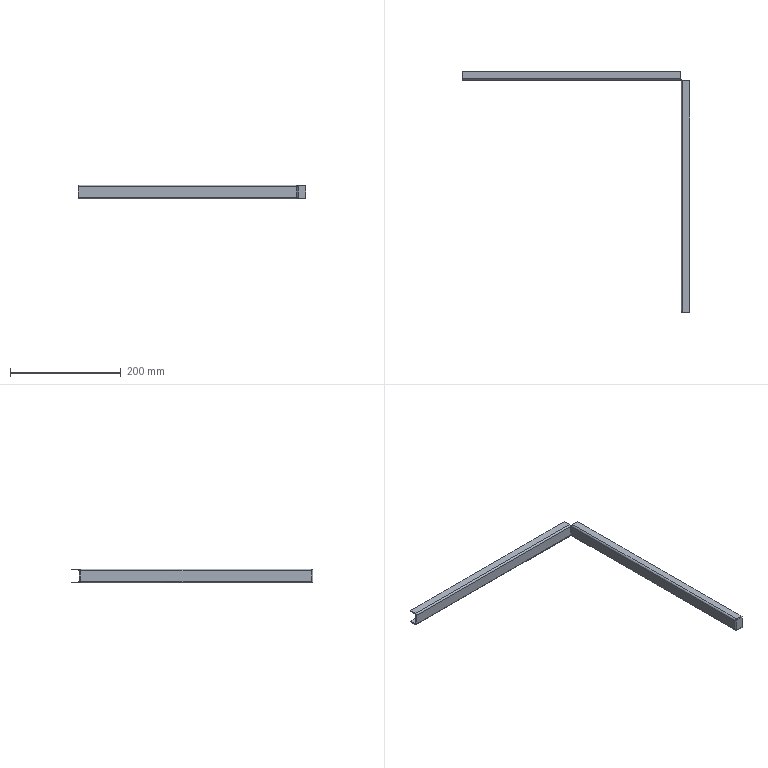Part | NX | features solid 2 | 1 solid | 50 faces | box 411 x 436 x 25 mm | volume 63952 mm3 | plane 38 | cylinder 12 | commonest cylinder face diameters 3 x6 6 x6
STEP:
#1=CARTESIAN_POINT('',(1095.5,89.,905.9));
#2=VERTEX_POINT('',#1);
#3=CARTESIAN_POINT('',(1095.5,89.,884.1));
#4=VERTEX_POINT('',#3);
#5=CARTESIAN_POINT('',(1095.5,89.,904.5));
#6=DIRECTION('',(0.,0.,-1.));
#7=VECTOR('',#6,1000.);
#8=LINE('',#5,#7);
#9=EDGE_CURVE('',#2,#4,#8,.T.);
#10=ORIENTED_EDGE('',*,*,#9,.F.);
#11=CARTESIAN_POINT('',(1108.5,89.,905.9));
#12=VERTEX_POINT('',#11);
#13=CARTESIAN_POINT('',(1093.851,89.,905.9));
#14=DIRECTION('',(-1.,0.,0.));
#15=VECTOR('',#14,1000.);
#16=LINE('',#13,#15);
#17=EDGE_CURVE('',#12,#2,#16,.T.);
#18=ORIENTED_EDGE('',*,*,#17,.F.);
#19=CARTESIAN_POINT('',(1108.5,89.,884.1));
#20=VERTEX_POINT('',#19);
#21=CARTESIAN_POINT('',(1108.5,89.,885.5));
#22=DIRECTION('',(0.,0.,1.));
#23=VECTOR('',#22,1000.);
#24=LINE('',#21,#23);
#25=EDGE_CURVE('',#20,#12,#24,.T.);
#26=ORIENTED_EDGE('',*,*,#25,.F.);
#27=CARTESIAN_POINT('',(1093.851,89.,884.1));
#28=DIRECTION('',(1.,0.,0.));
#29=VECTOR('',#28,1000.);
#30=LINE('',#27,#29);
#31=EDGE_CURVE('',#4,#20,#30,.T.);
#32=ORIENTED_EDGE('',*,*,#31,.F.);
#33=EDGE_LOOP('',(#10,#18,#26,#32));
#34=FACE_BOUND('',#33,.T.);
#35=CARTESIAN_POINT('',(895.,89.,895.));
#36=DIRECTION('',(0.,-1.,0.));
#37=DIRECTION('',(-1.,0.,0.));
#38=AXIS2_PLACEMENT_3D('',#35,#36,#37);
#39=PLANE('',#38);
#40=ADVANCED_FACE('',(#34),#39,.F.);
#41=CARTESIAN_POINT('',(1108.5,87.5,905.9));
#42=VERTEX_POINT('',#41);
#43=CARTESIAN_POINT('',(1095.5,87.5,905.9));
#44=VERTEX_POINT('',#43);
#45=CARTESIAN_POINT('',(1093.851,87.5,905.9));
#46=DIRECTION('',(-1.,0.,0.));
#47=VECTOR('',#46,1000.);
#48=LINE('',#45,#47);
#49=EDGE_CURVE('',#42,#44,#48,.T.);
#50=ORIENTED_EDGE('',*,*,#49,.T.);
#51=CARTESIAN_POINT('',(1095.5,87.5,884.1));
#52=VERTEX_POINT('',#51);
#53=CARTESIAN_POINT('',(1095.5,87.5,904.5));
#54=DIRECTION('',(0.,0.,-1.));
#55=VECTOR('',#54,1000.);
#56=LINE('',#53,#55);
#57=EDGE_CURVE('',#44,#52,#56,.T.);
#58=ORIENTED_EDGE('',*,*,#57,.T.);
#59=CARTESIAN_POINT('',(1108.5,87.5,884.1));
#60=VERTEX_POINT('',#59);
#61=CARTESIAN_POINT('',(1093.851,87.5,884.1));
#62=DIRECTION('',(1.,0.,0.));
#63=VECTOR('',#62,1000.);
#64=LINE('',#61,#63);
#65=EDGE_CURVE('',#52,#60,#64,.T.);
#66=ORIENTED_EDGE('',*,*,#65,.T.);
#67=CARTESIAN_POINT('',(1108.5,87.5,885.5));
#68=DIRECTION('',(0.,0.,1.));
#69=VECTOR('',#68,1000.);
#70=LINE('',#67,#69);
#71=EDGE_CURVE('',#60,#42,#70,.T.);
#72=ORIENTED_EDGE('',*,*,#71,.T.);
#73=EDGE_LOOP('',(#50,#58,#66,#72));
#74=FACE_BOUND('',#73,.T.);
#75=CARTESIAN_POINT('',(895.,87.5,895.));
#76=DIRECTION('',(0.,-1.,0.));
#77=DIRECTION('',(-1.,0.,0.));
#78=AXIS2_PLACEMENT_3D('',#75,#76,#77);
#79=PLANE('',#78);
#80=ADVANCED_FACE('',(#74),#79,.T.);
#81=ORIENTED_EDGE('',*,*,#25,.T.);
#82=CARTESIAN_POINT('',(1108.5,87.5,905.9));
#83=DIRECTION('',(0.,1.,0.));
#84=VECTOR('',#83,1000.);
#85=LINE('',#82,#84);
#86=EDGE_CURVE('',#42,#12,#85,.T.);
#87=ORIENTED_EDGE('',*,*,#86,.F.);
#88=ORIENTED_EDGE('',*,*,#71,.F.);
#89=CARTESIAN_POINT('',(1108.5,87.5,884.1));
#90=DIRECTION('',(0.,1.,0.));
#91=VECTOR('',#90,1000.);
#92=LINE('',#89,#91);
#93=EDGE_CURVE('',#60,#20,#92,.T.);
#94=ORIENTED_EDGE('',*,*,#93,.T.);
#95=EDGE_LOOP('',(#81,#87,#88,#94));
#96=FACE_BOUND('',#95,.T.);
#97=CARTESIAN_POINT('',(1108.5,87.5,885.5));
#98=DIRECTION('',(-1.,0.,0.));
#99=DIRECTION('',(0.,0.,1.));
#100=AXIS2_PLACEMENT_3D('',#97,#98,#99);
#101=PLANE('',#100);
#102=ADVANCED_FACE('',(#96),#101,.F.);
#103=CARTESIAN_POINT('',(1094.,90.5,885.5));
#104=VERTEX_POINT('',#103);
#105=CARTESIAN_POINT('',(1095.5,89.,884.1));
#106=CARTESIAN_POINT('',(1094.621,89.,884.1));
#107=CARTESIAN_POINT('',(1094.,89.621,884.68));
#108=CARTESIAN_POINT('',(1094.,90.5,885.5));
#109=(BOUNDED_CURVE()B_SPLINE_CURVE(3,(#105,#106,#107,#108),.UNSPECIFIED.,.F.,.F.)B_SPLINE_CURVE_WITH_KNOTS((4,4),(3.142,4.712),.PIECEWISE_BEZIER_KNOTS.)CURVE()GEOMETRIC_REPRESENTATION_ITEM()RATIONAL_B_SPLINE_CURVE((1.,0.8047,0.8047,1.))REPRESENTATION_ITEM(''));
#110=EDGE_CURVE('',#4,#104,#109,.T.);
#111=ORIENTED_EDGE('',*,*,#110,.F.);
#112=CARTESIAN_POINT('',(1092.902,89.,884.1));
#113=VERTEX_POINT('',#112);
#114=CARTESIAN_POINT('',(2092.5,89.,884.1));
#115=DIRECTION('',(1.,0.,0.));
#116=VECTOR('',#115,1000.);
#117=LINE('',#114,#116);
#118=EDGE_CURVE('',#113,#4,#117,.T.);
#119=ORIENTED_EDGE('',*,*,#118,.F.);
#120=CARTESIAN_POINT('',(1092.5,90.5,885.5));
#121=VERTEX_POINT('',#120);
#122=CARTESIAN_POINT('',(1092.902,89.,884.1));
#123=CARTESIAN_POINT('',(1092.637,89.459,884.528));
#124=CARTESIAN_POINT('',(1092.5,89.97,885.006));
#125=CARTESIAN_POINT('',(1092.5,90.5,885.5));
#126=(BOUNDED_CURVE()B_SPLINE_CURVE(3,(#122,#123,#124,#125),.UNSPECIFIED.,.F.,.F.)B_SPLINE_CURVE_WITH_KNOTS((4,4),(4.189,4.712),.PIECEWISE_BEZIER_KNOTS.)CURVE()GEOMETRIC_REPRESENTATION_ITEM()RATIONAL_B_SPLINE_CURVE((1.,0.9773,0.9773,1.))REPRESENTATION_ITEM(''));
#127=EDGE_CURVE('',#113,#121,#126,.T.);
#128=ORIENTED_EDGE('',*,*,#127,.T.);
#129=CARTESIAN_POINT('',(1094.,90.5,885.5));
#130=DIRECTION('',(-1.,0.,0.));
#131=VECTOR('',#130,1000.);
#132=LINE('',#129,#131);
#133=EDGE_CURVE('',#104,#121,#132,.T.);
#134=ORIENTED_EDGE('',*,*,#133,.F.);
#135=EDGE_LOOP('',(#111,#119,#128,#134));
#136=FACE_BOUND('',#135,.T.);
#137=CARTESIAN_POINT('',(92.5,821.555,1567.818));
#138=DIRECTION('',(0.,-0.6823,0.7311));
#139=DIRECTION('',(-1.,0.,0.));
#140=AXIS2_PLACEMENT_3D('',#137,#138,#139);
#141=PLANE('',#140);
#142=ADVANCED_FACE('',(#136),#141,.F.);
#143=ORIENTED_EDGE('',*,*,#118,.T.);
#144=ORIENTED_EDGE('',*,*,#31,.T.);
#145=ORIENTED_EDGE('',*,*,#93,.F.);
#146=ORIENTED_EDGE('',*,*,#65,.F.);
#147=CARTESIAN_POINT('',(1095.5,90.5,884.1));
#148=DIRECTION('',(0.,0.,-1.));
#149=DIRECTION('',(0.,1.,0.));
#150=AXIS2_PLACEMENT_3D('',#147,#148,#149);
#151=CIRCLE('',#150,3.);
#152=EDGE_CURVE('',#52,#113,#151,.T.);
#153=ORIENTED_EDGE('',*,*,#152,.T.);
#154=EDGE_LOOP('',(#143,#144,#145,#146,#153));
#155=FACE_BOUND('',#154,.T.);
#156=CARTESIAN_POINT('',(92.5,89.,884.1));
#157=DIRECTION('',(0.,0.,1.));
#158=DIRECTION('',(0.,-1.,0.));
#159=AXIS2_PLACEMENT_3D('',#156,#157,#158);
#160=PLANE('',#159);
#161=ADVANCED_FACE('',(#155),#160,.F.);
#162=CARTESIAN_POINT('',(1092.902,89.,905.9));
#163=VERTEX_POINT('',#162);
#164=CARTESIAN_POINT('',(1092.5,90.5,904.5));
#165=VERTEX_POINT('',#164);
#166=CARTESIAN_POINT('',(1092.902,89.,905.9));
#167=CARTESIAN_POINT('',(1092.637,89.459,905.472));
#168=CARTESIAN_POINT('',(1092.5,89.97,904.994));
#169=CARTESIAN_POINT('',(1092.5,90.5,904.5));
#170=(BOUNDED_CURVE()B_SPLINE_CURVE(3,(#166,#167,#168,#169),.UNSPECIFIED.,.F.,.F.)B_SPLINE_CURVE_WITH_KNOTS((4,4),(1.047,1.571),.PIECEWISE_BEZIER_KNOTS.)CURVE()GEOMETRIC_REPRESENTATION_ITEM()RATIONAL_B_SPLINE_CURVE((1.,0.9773,0.9773,1.))REPRESENTATION_ITEM(''));
#171=EDGE_CURVE('',#163,#165,#170,.T.);
#172=ORIENTED_EDGE('',*,*,#171,.F.);
#173=CARTESIAN_POINT('',(2092.5,89.,905.9));
#174=DIRECTION('',(1.,0.,0.));
#175=VECTOR('',#174,1000.);
#176=LINE('',#173,#175);
#177=EDGE_CURVE('',#163,#2,#176,.T.);
#178=ORIENTED_EDGE('',*,*,#177,.T.);
#179=CARTESIAN_POINT('',(1094.,90.5,904.5));
#180=VERTEX_POINT('',#179);
#181=CARTESIAN_POINT('',(1095.5,89.,905.9));
#182=CARTESIAN_POINT('',(1094.621,89.,905.9));
#183=CARTESIAN_POINT('',(1094.,89.621,905.32));
#184=CARTESIAN_POINT('',(1094.,90.5,904.5));
#185=(BOUNDED_CURVE()B_SPLINE_CURVE(3,(#181,#182,#183,#184),.UNSPECIFIED.,.F.,.F.)B_SPLINE_CURVE_WITH_KNOTS((4,4),(0.,1.571),.PIECEWISE_BEZIER_KNOTS.)CURVE()GEOMETRIC_REPRESENTATION_ITEM()RATIONAL_B_SPLINE_CURVE((1.,0.8047,0.8047,1.))REPRESENTATION_ITEM(''));
#186=EDGE_CURVE('',#2,#180,#185,.T.);
#187=ORIENTED_EDGE('',*,*,#186,.T.);
#188=CARTESIAN_POINT('',(1094.,90.5,904.5));
#189=DIRECTION('',(-1.,0.,0.));
#190=VECTOR('',#189,1000.);
#191=LINE('',#188,#190);
#192=EDGE_CURVE('',#180,#165,#191,.T.);
#193=ORIENTED_EDGE('',*,*,#192,.T.);
#194=EDGE_LOOP('',(#172,#178,#187,#193));
#195=FACE_BOUND('',#194,.T.);
#196=CARTESIAN_POINT('',(92.5,821.555,222.182));
#197=DIRECTION('',(0.,0.6823,0.7311));
#198=DIRECTION('',(1.,0.,0.));
#199=AXIS2_PLACEMENT_3D('',#196,#197,#198);
#200=PLANE('',#199);
#201=ADVANCED_FACE('',(#195),#200,.T.);
#202=ORIENTED_EDGE('',*,*,#127,.F.);
#203=ORIENTED_EDGE('',*,*,#152,.F.);
#204=ORIENTED_EDGE('',*,*,#57,.F.);
#205=CARTESIAN_POINT('',(1095.5,90.5,905.9));
#206=DIRECTION('',(0.,0.,-1.));
#207=DIRECTION('',(0.,1.,0.));
#208=AXIS2_PLACEMENT_3D('',#205,#206,#207);
#209=CIRCLE('',#208,3.);
#210=EDGE_CURVE('',#44,#163,#209,.T.);
#211=ORIENTED_EDGE('',*,*,#210,.T.);
#212=ORIENTED_EDGE('',*,*,#171,.T.);
#213=CARTESIAN_POINT('',(1092.5,90.5,885.5));
#214=DIRECTION('',(0.,0.,1.));
#215=VECTOR('',#214,1000.);
#216=LINE('',#213,#215);
#217=EDGE_CURVE('',#121,#165,#216,.T.);
#218=ORIENTED_EDGE('',*,*,#217,.F.);
#219=EDGE_LOOP('',(#202,#203,#204,#211,#212,#218));
#220=FACE_BOUND('',#219,.T.);
#221=CARTESIAN_POINT('',(1095.5,90.5,885.5));
#222=DIRECTION('',(0.,0.,1.));
#223=DIRECTION('',(1.,0.,0.));
#224=AXIS2_PLACEMENT_3D('',#221,#222,#223);
#225=CYLINDRICAL_SURFACE('',#224,3.);
#226=ADVANCED_FACE('',(#220),#225,.T.);
#227=ORIENTED_EDGE('',*,*,#210,.F.);
#228=ORIENTED_EDGE('',*,*,#49,.F.);
#229=ORIENTED_EDGE('',*,*,#86,.T.);
#230=ORIENTED_EDGE('',*,*,#17,.T.);
#231=ORIENTED_EDGE('',*,*,#177,.F.);
#232=EDGE_LOOP('',(#227,#228,#229,#230,#231));
#233=FACE_BOUND('',#232,.T.);
#234=CARTESIAN_POINT('',(92.5,89.,905.9));
#235=DIRECTION('',(0.,0.,1.));
#236=DIRECTION('',(0.,-1.,0.));
#237=AXIS2_PLACEMENT_3D('',#234,#235,#236);
#238=PLANE('',#237);
#239=ADVANCED_FACE('',(#233),#238,.T.);
#240=ORIENTED_EDGE('',*,*,#9,.T.);
#241=ORIENTED_EDGE('',*,*,#110,.T.);
#242=CARTESIAN_POINT('',(1094.,90.5,885.5));
#243=DIRECTION('',(0.,0.,1.));
#244=VECTOR('',#243,1000.);
#245=LINE('',#242,#244);
#246=EDGE_CURVE('',#104,#180,#245,.T.);
#247=ORIENTED_EDGE('',*,*,#246,.T.);
#248=ORIENTED_EDGE('',*,*,#186,.F.);
#249=EDGE_LOOP('',(#240,#241,#247,#248));
#250=FACE_BOUND('',#249,.T.);
#251=CARTESIAN_POINT('',(1095.5,90.5,885.5));
#252=DIRECTION('',(0.,0.,1.));
#253=DIRECTION('',(1.,0.,0.));
#254=AXIS2_PLACEMENT_3D('',#251,#252,#253);
#255=CYLINDRICAL_SURFACE('',#254,1.5);
#256=ADVANCED_FACE('',(#250),#255,.F.);
#257=CARTESIAN_POINT('',(1108.5,506.,884.));
#258=VERTEX_POINT('',#257);
#259=CARTESIAN_POINT('',(1095.5,506.,884.));
#260=VERTEX_POINT('',#259);
#261=CARTESIAN_POINT('',(1108.5,506.,884.));
#262=DIRECTION('',(-1.,0.,0.));
#263=VECTOR('',#262,1000.);
#264=LINE('',#261,#263);
#265=EDGE_CURVE('',#258,#260,#264,.T.);
#266=ORIENTED_EDGE('',*,*,#265,.T.);
#267=CARTESIAN_POINT('',(1095.5,89.1,884.));
#268=VERTEX_POINT('',#267);
#269=CARTESIAN_POINT('',(1095.5,87.5,884.));
#270=DIRECTION('',(0.,1.,0.));
#271=VECTOR('',#270,1000.);
#272=LINE('',#269,#271);
#273=EDGE_CURVE('',#268,#260,#272,.T.);
#274=ORIENTED_EDGE('',*,*,#273,.F.);
#275=CARTESIAN_POINT('',(1095.5,87.5,884.));
#276=VERTEX_POINT('',#275);
#277=CARTESIAN_POINT('',(1095.5,87.5,884.));
#278=DIRECTION('',(0.,1.,0.));
#279=VECTOR('',#278,1000.);
#280=LINE('',#277,#279);
#281=EDGE_CURVE('',#276,#268,#280,.T.);
#282=ORIENTED_EDGE('',*,*,#281,.F.);
#283=CARTESIAN_POINT('',(1108.5,87.5,884.));
#284=VERTEX_POINT('',#283);
#285=CARTESIAN_POINT('',(1108.5,87.5,884.));
#286=DIRECTION('',(-1.,0.,0.));
#287=VECTOR('',#286,1000.);
#288=LINE('',#285,#287);
#289=EDGE_CURVE('',#284,#276,#288,.T.);
#290=ORIENTED_EDGE('',*,*,#289,.F.);
#291=CARTESIAN_POINT('',(1108.5,87.5,884.));
#292=DIRECTION('',(0.,1.,0.));
#293=VECTOR('',#292,1000.);
#294=LINE('',#291,#293);
#295=EDGE_CURVE('',#284,#258,#294,.T.);
#296=ORIENTED_EDGE('',*,*,#295,.T.);
#297=EDGE_LOOP('',(#266,#274,#282,#290,#296));
#298=FACE_BOUND('',#297,.T.);
#299=CARTESIAN_POINT('',(1108.5,87.5,884.));
#300=DIRECTION('',(0.,0.,-1.));
#301=DIRECTION('',(-1.,0.,0.));
#302=AXIS2_PLACEMENT_3D('',#299,#300,#301);
#303=PLANE('',#302);
#304=ADVANCED_FACE('',(#298),#303,.F.);
#305=CARTESIAN_POINT('',(1108.5,506.,882.5));
#306=VERTEX_POINT('',#305);
#307=CARTESIAN_POINT('',(1095.5,506.,882.5));
#308=VERTEX_POINT('',#307);
#309=CARTESIAN_POINT('',(1108.5,506.,882.5));
#310=DIRECTION('',(-1.,0.,0.));
#311=VECTOR('',#310,1000.);
#312=LINE('',#309,#311);
#313=EDGE_CURVE('',#306,#308,#312,.T.);
#314=ORIENTED_EDGE('',*,*,#313,.F.);
#315=CARTESIAN_POINT('',(1108.5,87.5,882.5));
#316=VERTEX_POINT('',#315);
#317=CARTESIAN_POINT('',(1108.5,87.5,882.5));
#318=DIRECTION('',(0.,1.,0.));
#319=VECTOR('',#318,1000.);
#320=LINE('',#317,#319);
#321=EDGE_CURVE('',#316,#306,#320,.T.);
#322=ORIENTED_EDGE('',*,*,#321,.F.);
#323=CARTESIAN_POINT('',(1095.5,87.5,882.5));
#324=VERTEX_POINT('',#323);
#325=CARTESIAN_POINT('',(1108.5,87.5,882.5));
#326=DIRECTION('',(-1.,0.,0.));
#327=VECTOR('',#326,1000.);
#328=LINE('',#325,#327);
#329=EDGE_CURVE('',#316,#324,#328,.T.);
#330=ORIENTED_EDGE('',*,*,#329,.T.);
#331=CARTESIAN_POINT('',(1095.5,89.1,882.5));
#332=VERTEX_POINT('',#331);
#333=CARTESIAN_POINT('',(1095.5,87.5,882.5));
#334=DIRECTION('',(0.,1.,0.));
#335=VECTOR('',#334,1000.);
#336=LINE('',#333,#335);
#337=EDGE_CURVE('',#324,#332,#336,.T.);
#338=ORIENTED_EDGE('',*,*,#337,.T.);
#339=CARTESIAN_POINT('',(1095.5,87.5,882.5));
#340=DIRECTION('',(0.,1.,0.));
#341=VECTOR('',#340,1000.);
#342=LINE('',#339,#341);
#343=EDGE_CURVE('',#332,#308,#342,.T.);
#344=ORIENTED_EDGE('',*,*,#343,.T.);
#345=EDGE_LOOP('',(#314,#322,#330,#338,#344));
#346=FACE_BOUND('',#345,.T.);
#347=CARTESIAN_POINT('',(1108.5,87.5,882.5));
#348=DIRECTION('',(0.,0.,-1.));
#349=DIRECTION('',(-1.,0.,0.));
#350=AXIS2_PLACEMENT_3D('',#347,#348,#349);
#351=PLANE('',#350);
#352=ADVANCED_FACE('',(#346),#351,.T.);
#353=CARTESIAN_POINT('',(1095.5,87.5,882.5));
#354=DIRECTION('',(0.,0.,1.));
#355=VECTOR('',#354,1000.);
#356=LINE('',#353,#355);
#357=EDGE_CURVE('',#324,#276,#356,.T.);
#358=ORIENTED_EDGE('',*,*,#357,.F.);
#359=ORIENTED_EDGE('',*,*,#329,.F.);
#360=CARTESIAN_POINT('',(1108.5,87.5,882.5));
#361=DIRECTION('',(0.,0.,-1.));
#362=VECTOR('',#361,1000.);
#363=LINE('',#360,#362);
#364=EDGE_CURVE('',#284,#316,#363,.T.);
#365=ORIENTED_EDGE('',*,*,#364,.F.);
#366=ORIENTED_EDGE('',*,*,#289,.T.);
#367=EDGE_LOOP('',(#358,#359,#365,#366));
#368=FACE_BOUND('',#367,.T.);
#369=CARTESIAN_POINT('',(1092.5,87.5,882.5));
#370=DIRECTION('',(0.,1.,0.));
#371=DIRECTION('',(1.,0.,0.));
#372=AXIS2_PLACEMENT_3D('',#369,#370,#371);
#373=PLANE('',#372);
#374=ADVANCED_FACE('',(#368),#373,.F.);
#375=ORIENTED_EDGE('',*,*,#295,.F.);
#376=ORIENTED_EDGE('',*,*,#364,.T.);
#377=ORIENTED_EDGE('',*,*,#321,.T.);
#378=CARTESIAN_POINT('',(1108.5,506.,882.5));
#379=DIRECTION('',(0.,0.,-1.));
#380=VECTOR('',#379,1000.);
#381=LINE('',#378,#380);
#382=EDGE_CURVE('',#258,#306,#381,.T.);
#383=ORIENTED_EDGE('',*,*,#382,.F.);
#384=EDGE_LOOP('',(#375,#376,#377,#383));
#385=FACE_BOUND('',#384,.T.);
#386=CARTESIAN_POINT('',(1108.5,87.5,882.5));
#387=DIRECTION('',(-1.,0.,0.));
#388=DIRECTION('',(0.,1.,0.));
#389=AXIS2_PLACEMENT_3D('',#386,#387,#388);
#390=PLANE('',#389);
#391=ADVANCED_FACE('',(#385),#390,.F.);
#392=ORIENTED_EDGE('',*,*,#281,.T.);
#393=CARTESIAN_POINT('',(1095.5,89.1,895.));
#394=DIRECTION('',(0.,0.,-1.));
#395=VECTOR('',#394,1000.);
#396=LINE('',#393,#395);
#397=EDGE_CURVE('',#268,#332,#396,.T.);
#398=ORIENTED_EDGE('',*,*,#397,.T.);
#399=ORIENTED_EDGE('',*,*,#337,.F.);
#400=ORIENTED_EDGE('',*,*,#357,.T.);
#401=EDGE_LOOP('',(#392,#398,#399,#400));
#402=FACE_BOUND('',#401,.T.);
#403=CARTESIAN_POINT('',(1095.5,87.5,882.5));
#404=DIRECTION('',(1.,0.,0.));
#405=DIRECTION('',(0.,-1.,0.));
#406=AXIS2_PLACEMENT_3D('',#403,#404,#405);
#407=PLANE('',#406);
#408=ADVANCED_FACE('',(#402),#407,.F.);
#409=CARTESIAN_POINT('',(1092.902,89.1,884.));
#410=VERTEX_POINT('',#409);
#411=CARTESIAN_POINT('',(1095.5,89.1,885.5));
#412=DIRECTION('',(0.,1.,0.));
#413=DIRECTION('',(0.,0.,1.));
#414=AXIS2_PLACEMENT_3D('',#411,#412,#413);
#415=CIRCLE('',#414,3.);
#416=EDGE_CURVE('',#332,#410,#415,.T.);
#417=ORIENTED_EDGE('',*,*,#416,.F.);
#418=ORIENTED_EDGE('',*,*,#397,.F.);
#419=CARTESIAN_POINT('',(2092.5,89.1,884.));
#420=DIRECTION('',(1.,0.,0.));
#421=VECTOR('',#420,1000.);
#422=LINE('',#419,#421);
#423=EDGE_CURVE('',#410,#268,#422,.T.);
#424=ORIENTED_EDGE('',*,*,#423,.F.);
#425=EDGE_LOOP('',(#417,#418,#424));
#426=FACE_BOUND('',#425,.T.);
#427=CARTESIAN_POINT('',(92.5,89.1,884.));
#428=DIRECTION('',(0.,-1.,0.));
#429=DIRECTION('',(-1.,0.,0.));
#430=AXIS2_PLACEMENT_3D('',#427,#428,#429);
#431=PLANE('',#430);
#432=ADVANCED_FACE('',(#426),#431,.T.);
#433=CARTESIAN_POINT('',(1092.902,89.1,884.));
#434=CARTESIAN_POINT('',(1092.637,89.528,884.459));
#435=CARTESIAN_POINT('',(1092.5,90.006,884.97));
#436=CARTESIAN_POINT('',(1092.5,90.5,885.5));
#437=(BOUNDED_CURVE()B_SPLINE_CURVE(3,(#433,#434,#435,#436),.UNSPECIFIED.,.F.,.F.)B_SPLINE_CURVE_WITH_KNOTS((4,4),(4.189,4.712),.PIECEWISE_BEZIER_KNOTS.)CURVE()GEOMETRIC_REPRESENTATION_ITEM()RATIONAL_B_SPLINE_CURVE((1.,0.9773,0.9773,1.))REPRESENTATION_ITEM(''));
#438=EDGE_CURVE('',#410,#121,#437,.T.);
#439=ORIENTED_EDGE('',*,*,#438,.F.);
#440=ORIENTED_EDGE('',*,*,#423,.T.);
#441=CARTESIAN_POINT('',(1095.5,89.1,884.));
#442=CARTESIAN_POINT('',(1094.621,89.1,884.));
#443=CARTESIAN_POINT('',(1094.,89.68,884.621));
#444=CARTESIAN_POINT('',(1094.,90.5,885.5));
#445=(BOUNDED_CURVE()B_SPLINE_CURVE(3,(#441,#442,#443,#444),.UNSPECIFIED.,.F.,.F.)B_SPLINE_CURVE_WITH_KNOTS((4,4),(3.142,4.712),.PIECEWISE_BEZIER_KNOTS.)CURVE()GEOMETRIC_REPRESENTATION_ITEM()RATIONAL_B_SPLINE_CURVE((1.,0.8047,0.8047,1.))REPRESENTATION_ITEM(''));
#446=EDGE_CURVE('',#268,#104,#445,.T.);
#447=ORIENTED_EDGE('',*,*,#446,.T.);
#448=ORIENTED_EDGE('',*,*,#133,.T.);
#449=EDGE_LOOP('',(#439,#440,#447,#448));
#450=FACE_BOUND('',#449,.T.);
#451=CARTESIAN_POINT('',(92.5,772.818,1616.555));
#452=DIRECTION('',(0.,-0.7311,0.6823));
#453=DIRECTION('',(-1.,0.,0.));
#454=AXIS2_PLACEMENT_3D('',#451,#452,#453);
#455=PLANE('',#454);
#456=ADVANCED_FACE('',(#450),#455,.T.);
#457=CARTESIAN_POINT('',(1094.,506.,885.5));
#458=VERTEX_POINT('',#457);
#459=CARTESIAN_POINT('',(1095.5,506.,885.5));
#460=DIRECTION('',(0.,-1.,0.));
#461=DIRECTION('',(0.,0.,-1.));
#462=AXIS2_PLACEMENT_3D('',#459,#460,#461);
#463=CIRCLE('',#462,1.5);
#464=EDGE_CURVE('',#458,#260,#463,.T.);
#465=ORIENTED_EDGE('',*,*,#464,.T.);
#466=ORIENTED_EDGE('',*,*,#265,.F.);
#467=ORIENTED_EDGE('',*,*,#382,.T.);
#468=ORIENTED_EDGE('',*,*,#313,.T.);
#469=CARTESIAN_POINT('',(1092.5,506.,885.5));
#470=VERTEX_POINT('',#469);
#471=CARTESIAN_POINT('',(1095.5,506.,885.5));
#472=DIRECTION('',(0.,-1.,0.));
#473=DIRECTION('',(1.,0.,0.));
#474=AXIS2_PLACEMENT_3D('',#471,#472,#473);
#475=CIRCLE('',#474,3.);
#476=EDGE_CURVE('',#470,#308,#475,.T.);
#477=ORIENTED_EDGE('',*,*,#476,.F.);
#478=CARTESIAN_POINT('',(1092.5,506.,885.5));
#479=DIRECTION('',(-1.,0.,0.));
#480=VECTOR('',#479,1000.);
#481=LINE('',#478,#480);
#482=EDGE_CURVE('',#458,#470,#481,.T.);
#483=ORIENTED_EDGE('',*,*,#482,.F.);
#484=EDGE_LOOP('',(#465,#466,#467,#468,#477,#483));
#485=FACE_BOUND('',#484,.T.);
#486=CARTESIAN_POINT('',(1108.5,506.,882.5));
#487=DIRECTION('',(0.,-1.,0.));
#488=DIRECTION('',(-1.,0.,0.));
#489=AXIS2_PLACEMENT_3D('',#486,#487,#488);
#490=PLANE('',#489);
#491=ADVANCED_FACE('',(#485),#490,.F.);
#492=ORIENTED_EDGE('',*,*,#446,.F.);
#493=ORIENTED_EDGE('',*,*,#273,.T.);
#494=ORIENTED_EDGE('',*,*,#464,.F.);
#495=CARTESIAN_POINT('',(1094.,506.,885.5));
#496=DIRECTION('',(0.,-1.,0.));
#497=VECTOR('',#496,1000.);
#498=LINE('',#495,#497);
#499=EDGE_CURVE('',#458,#104,#498,.T.);
#500=ORIENTED_EDGE('',*,*,#499,.T.);
#501=EDGE_LOOP('',(#492,#493,#494,#500));
#502=FACE_BOUND('',#501,.T.);
#503=CARTESIAN_POINT('',(1095.5,506.,885.5));
#504=DIRECTION('',(0.,1.,0.));
#505=DIRECTION('',(1.,0.,0.));
#506=AXIS2_PLACEMENT_3D('',#503,#504,#505);
#507=CYLINDRICAL_SURFACE('',#506,1.5);
#508=ADVANCED_FACE('',(#502),#507,.F.);
#509=ORIENTED_EDGE('',*,*,#416,.T.);
#510=ORIENTED_EDGE('',*,*,#438,.T.);
#511=CARTESIAN_POINT('',(1092.5,87.5,885.5));
#512=DIRECTION('',(0.,-1.,0.));
#513=VECTOR('',#512,1000.);
#514=LINE('',#511,#513);
#515=EDGE_CURVE('',#470,#121,#514,.T.);
#516=ORIENTED_EDGE('',*,*,#515,.F.);
#517=ORIENTED_EDGE('',*,*,#476,.T.);
#518=ORIENTED_EDGE('',*,*,#343,.F.);
#519=EDGE_LOOP('',(#509,#510,#516,#517,#518));
#520=FACE_BOUND('',#519,.T.);
#521=CARTESIAN_POINT('',(1095.5,506.,885.5));
#522=DIRECTION('',(0.,1.,0.));
#523=DIRECTION('',(1.,0.,0.));
#524=AXIS2_PLACEMENT_3D('',#521,#522,#523);
#525=CYLINDRICAL_SURFACE('',#524,3.);
#526=ADVANCED_FACE('',(#520),#525,.T.);
#527=CARTESIAN_POINT('',(1095.5,506.,907.5));
#528=VERTEX_POINT('',#527);
#529=CARTESIAN_POINT('',(1108.5,506.,907.5));
#530=VERTEX_POINT('',#529);
#531=CARTESIAN_POINT('',(1092.5,506.,907.5));
#532=DIRECTION('',(1.,0.,0.));
#533=VECTOR('',#532,1000.);
#534=LINE('',#531,#533);
#535=EDGE_CURVE('',#528,#530,#534,.T.);
#536=ORIENTED_EDGE('',*,*,#535,.F.);
#537=CARTESIAN_POINT('',(1095.5,89.1,907.5));
#538=VERTEX_POINT('',#537);
#539=CARTESIAN_POINT('',(1095.5,87.5,907.5));
#540=DIRECTION('',(0.,1.,0.));
#541=VECTOR('',#540,1000.);
#542=LINE('',#539,#541);
#543=EDGE_CURVE('',#538,#528,#542,.T.);
#544=ORIENTED_EDGE('',*,*,#543,.F.);
#545=CARTESIAN_POINT('',(1095.5,87.5,907.5));
#546=VERTEX_POINT('',#545);
#547=CARTESIAN_POINT('',(1095.5,87.5,907.5));
#548=DIRECTION('',(0.,1.,0.));
#549=VECTOR('',#548,1000.);
#550=LINE('',#547,#549);
#551=EDGE_CURVE('',#546,#538,#550,.T.);
#552=ORIENTED_EDGE('',*,*,#551,.F.);
#553=CARTESIAN_POINT('',(1108.5,87.5,907.5));
#554=VERTEX_POINT('',#553);
#555=CARTESIAN_POINT('',(1092.5,87.5,907.5));
#556=DIRECTION('',(1.,0.,0.));
#557=VECTOR('',#556,1000.);
#558=LINE('',#555,#557);
#559=EDGE_CURVE('',#546,#554,#558,.T.);
#560=ORIENTED_EDGE('',*,*,#559,.T.);
#561=CARTESIAN_POINT('',(1108.5,87.5,907.5));
#562=DIRECTION('',(0.,1.,0.));
#563=VECTOR('',#562,1000.);
#564=LINE('',#561,#563);
#565=EDGE_CURVE('',#554,#530,#564,.T.);
#566=ORIENTED_EDGE('',*,*,#565,.T.);
#567=EDGE_LOOP('',(#536,#544,#552,#560,#566));
#568=FACE_BOUND('',#567,.T.);
#569=CARTESIAN_POINT('',(1092.5,87.5,907.5));
#570=DIRECTION('',(0.,0.,1.));
#571=DIRECTION('',(0.,-1.,0.));
#572=AXIS2_PLACEMENT_3D('',#569,#570,#571);
#573=PLANE('',#572);
#574=ADVANCED_FACE('',(#568),#573,.T.);
#575=CARTESIAN_POINT('',(1095.5,506.,906.));
#576=VERTEX_POINT('',#575);
#577=CARTESIAN_POINT('',(1108.5,506.,906.));
#578=VERTEX_POINT('',#577);
#579=CARTESIAN_POINT('',(1092.5,506.,906.));
#580=DIRECTION('',(1.,0.,0.));
#581=VECTOR('',#580,1000.);
#582=LINE('',#579,#581);
#583=EDGE_CURVE('',#576,#578,#582,.T.);
#584=ORIENTED_EDGE('',*,*,#583,.T.);
#585=CARTESIAN_POINT('',(1108.5,87.5,906.));
#586=VERTEX_POINT('',#585);
#587=CARTESIAN_POINT('',(1108.5,87.5,906.));
#588=DIRECTION('',(0.,1.,0.));
#589=VECTOR('',#588,1000.);
#590=LINE('',#587,#589);
#591=EDGE_CURVE('',#586,#578,#590,.T.);
#592=ORIENTED_EDGE('',*,*,#591,.F.);
#593=CARTESIAN_POINT('',(1095.5,87.5,906.));
#594=VERTEX_POINT('',#593);
#595=CARTESIAN_POINT('',(1092.5,87.5,906.));
#596=DIRECTION('',(1.,0.,0.));
#597=VECTOR('',#596,1000.);
#598=LINE('',#595,#597);
#599=EDGE_CURVE('',#594,#586,#598,.T.);
#600=ORIENTED_EDGE('',*,*,#599,.F.);
#601=CARTESIAN_POINT('',(1095.5,89.1,906.));
#602=VERTEX_POINT('',#601);
#603=CARTESIAN_POINT('',(1095.5,87.5,906.));
#604=DIRECTION('',(0.,1.,0.));
#605=VECTOR('',#604,1000.);
#606=LINE('',#603,#605);
#607=EDGE_CURVE('',#594,#602,#606,.T.);
#608=ORIENTED_EDGE('',*,*,#607,.T.);
#609=CARTESIAN_POINT('',(1095.5,87.5,906.));
#610=DIRECTION('',(0.,1.,0.));
#611=VECTOR('',#610,1000.);
#612=LINE('',#609,#611);
#613=EDGE_CURVE('',#602,#576,#612,.T.);
#614=ORIENTED_EDGE('',*,*,#613,.T.);
#615=EDGE_LOOP('',(#584,#592,#600,#608,#614));
#616=FACE_BOUND('',#615,.T.);
#617=CARTESIAN_POINT('',(1092.5,87.5,906.));
#618=DIRECTION('',(0.,0.,1.));
#619=DIRECTION('',(0.,-1.,0.));
#620=AXIS2_PLACEMENT_3D('',#617,#618,#619);
#621=PLANE('',#620);
#622=ADVANCED_FACE('',(#616),#621,.F.);
#623=ORIENTED_EDGE('',*,*,#551,.T.);
#624=CARTESIAN_POINT('',(1095.5,89.1,895.));
#625=DIRECTION('',(0.,0.,-1.));
#626=VECTOR('',#625,1000.);
#627=LINE('',#624,#626);
#628=EDGE_CURVE('',#538,#602,#627,.T.);
#629=ORIENTED_EDGE('',*,*,#628,.T.);
#630=ORIENTED_EDGE('',*,*,#607,.F.);
#631=CARTESIAN_POINT('',(1095.5,87.5,907.5));
#632=DIRECTION('',(0.,0.,-1.));
#633=VECTOR('',#632,1000.);
#634=LINE('',#631,#633);
#635=EDGE_CURVE('',#546,#594,#634,.T.);
#636=ORIENTED_EDGE('',*,*,#635,.F.);
#637=EDGE_LOOP('',(#623,#629,#630,#636));
#638=FACE_BOUND('',#637,.T.);
#639=CARTESIAN_POINT('',(1095.5,87.5,907.5));
#640=DIRECTION('',(-1.,0.,0.));
#641=DIRECTION('',(0.,0.,1.));
#642=AXIS2_PLACEMENT_3D('',#639,#640,#641);
#643=PLANE('',#642);
#644=ADVANCED_FACE('',(#638),#643,.T.);
#645=ORIENTED_EDGE('',*,*,#559,.F.);
#646=ORIENTED_EDGE('',*,*,#635,.T.);
#647=ORIENTED_EDGE('',*,*,#599,.T.);
#648=CARTESIAN_POINT('',(1108.5,87.5,907.5));
#649=DIRECTION('',(0.,0.,1.));
#650=VECTOR('',#649,1000.);
#651=LINE('',#648,#650);
#652=EDGE_CURVE('',#586,#554,#651,.T.);
#653=ORIENTED_EDGE('',*,*,#652,.T.);
#654=EDGE_LOOP('',(#645,#646,#647,#653));
#655=FACE_BOUND('',#654,.T.);
#656=CARTESIAN_POINT('',(1092.5,87.5,882.5));
#657=DIRECTION('',(0.,1.,0.));
#658=DIRECTION('',(1.,0.,0.));
#659=AXIS2_PLACEMENT_3D('',#656,#657,#658);
#660=PLANE('',#659);
#661=ADVANCED_FACE('',(#655),#660,.F.);
#662=ORIENTED_EDGE('',*,*,#652,.F.);
#663=ORIENTED_EDGE('',*,*,#591,.T.);
#664=CARTESIAN_POINT('',(1108.5,506.,907.5));
#665=DIRECTION('',(0.,0.,1.));
#666=VECTOR('',#665,1000.);
#667=LINE('',#664,#666);
#668=EDGE_CURVE('',#578,#530,#667,.T.);
#669=ORIENTED_EDGE('',*,*,#668,.T.);
#670=ORIENTED_EDGE('',*,*,#565,.F.);
#671=EDGE_LOOP('',(#662,#663,#669,#670));
#672=FACE_BOUND('',#671,.T.);
#673=CARTESIAN_POINT('',(1108.5,87.5,907.5));
#674=DIRECTION('',(1.,0.,0.));
#675=DIRECTION('',(0.,-1.,0.));
#676=AXIS2_PLACEMENT_3D('',#673,#674,#675);
#677=PLANE('',#676);
#678=ADVANCED_FACE('',(#672),#677,.T.);
#679=ORIENTED_EDGE('',*,*,#628,.F.);
#680=CARTESIAN_POINT('',(1092.902,89.1,906.));
#681=VERTEX_POINT('',#680);
#682=CARTESIAN_POINT('',(1095.5,89.1,904.5));
#683=DIRECTION('',(0.,-1.,0.));
#684=DIRECTION('',(0.,0.,-1.));
#685=AXIS2_PLACEMENT_3D('',#682,#683,#684);
#686=CIRCLE('',#685,3.);
#687=EDGE_CURVE('',#538,#681,#686,.T.);
#688=ORIENTED_EDGE('',*,*,#687,.T.);
#689=CARTESIAN_POINT('',(2092.5,89.1,906.));
#690=DIRECTION('',(1.,0.,0.));
#691=VECTOR('',#690,1000.);
#692=LINE('',#689,#691);
#693=EDGE_CURVE('',#681,#602,#692,.T.);
#694=ORIENTED_EDGE('',*,*,#693,.T.);
#695=EDGE_LOOP('',(#679,#688,#694));
#696=FACE_BOUND('',#695,.T.);
#697=CARTESIAN_POINT('',(92.5,89.1,906.));
#698=DIRECTION('',(0.,1.,0.));
#699=DIRECTION('',(1.,0.,0.));
#700=AXIS2_PLACEMENT_3D('',#697,#698,#699);
#701=PLANE('',#700);
#702=ADVANCED_FACE('',(#696),#701,.F.);
#703=CARTESIAN_POINT('',(1095.5,89.1,906.));
#704=CARTESIAN_POINT('',(1094.621,89.1,906.));
#705=CARTESIAN_POINT('',(1094.,89.68,905.379));
#706=CARTESIAN_POINT('',(1094.,90.5,904.5));
#707=(BOUNDED_CURVE()B_SPLINE_CURVE(3,(#703,#704,#705,#706),.UNSPECIFIED.,.F.,.F.)B_SPLINE_CURVE_WITH_KNOTS((4,4),(0.,1.571),.PIECEWISE_BEZIER_KNOTS.)CURVE()GEOMETRIC_REPRESENTATION_ITEM()RATIONAL_B_SPLINE_CURVE((1.,0.8047,0.8047,1.))REPRESENTATION_ITEM(''));
#708=EDGE_CURVE('',#602,#180,#707,.T.);
#709=ORIENTED_EDGE('',*,*,#708,.F.);
#710=ORIENTED_EDGE('',*,*,#693,.F.);
#711=CARTESIAN_POINT('',(1092.902,89.1,906.));
#712=CARTESIAN_POINT('',(1092.637,89.528,905.541));
#713=CARTESIAN_POINT('',(1092.5,90.006,905.03));
#714=CARTESIAN_POINT('',(1092.5,90.5,904.5));
#715=(BOUNDED_CURVE()B_SPLINE_CURVE(3,(#711,#712,#713,#714),.UNSPECIFIED.,.F.,.F.)B_SPLINE_CURVE_WITH_KNOTS((4,4),(1.047,1.571),.PIECEWISE_BEZIER_KNOTS.)CURVE()GEOMETRIC_REPRESENTATION_ITEM()RATIONAL_B_SPLINE_CURVE((1.,0.9773,0.9773,1.))REPRESENTATION_ITEM(''));
#716=EDGE_CURVE('',#681,#165,#715,.T.);
#717=ORIENTED_EDGE('',*,*,#716,.T.);
#718=ORIENTED_EDGE('',*,*,#192,.F.);
#719=EDGE_LOOP('',(#709,#710,#717,#718));
#720=FACE_BOUND('',#719,.T.);
#721=CARTESIAN_POINT('',(92.5,772.818,173.445));
#722=DIRECTION('',(0.,0.7311,0.6823));
#723=DIRECTION('',(1.,0.,0.));
#724=AXIS2_PLACEMENT_3D('',#721,#722,#723);
#725=PLANE('',#724);
#726=ADVANCED_FACE('',(#720),#725,.F.);
#727=ORIENTED_EDGE('',*,*,#716,.F.);
#728=ORIENTED_EDGE('',*,*,#687,.F.);
#729=ORIENTED_EDGE('',*,*,#543,.T.);
#730=CARTESIAN_POINT('',(1092.5,506.,904.5));
#731=VERTEX_POINT('',#730);
#732=CARTESIAN_POINT('',(1095.5,506.,904.5));
#733=DIRECTION('',(0.,-1.,0.));
#734=DIRECTION('',(1.,0.,0.));
#735=AXIS2_PLACEMENT_3D('',#732,#733,#734);
#736=CIRCLE('',#735,3.);
#737=EDGE_CURVE('',#528,#731,#736,.T.);
#738=ORIENTED_EDGE('',*,*,#737,.T.);
#739=CARTESIAN_POINT('',(1092.5,506.,904.5));
#740=DIRECTION('',(0.,1.,0.));
#741=VECTOR('',#740,1000.);
#742=LINE('',#739,#741);
#743=EDGE_CURVE('',#165,#731,#742,.T.);
#744=ORIENTED_EDGE('',*,*,#743,.F.);
#745=EDGE_LOOP('',(#727,#728,#729,#738,#744));
#746=FACE_BOUND('',#745,.T.);
#747=CARTESIAN_POINT('',(1095.5,87.5,904.5));
#748=DIRECTION('',(0.,-1.,0.));
#749=DIRECTION('',(1.,0.,0.));
#750=AXIS2_PLACEMENT_3D('',#747,#748,#749);
#751=CYLINDRICAL_SURFACE('',#750,3.);
#752=ADVANCED_FACE('',(#746),#751,.T.);
#753=ORIENTED_EDGE('',*,*,#737,.F.);
#754=ORIENTED_EDGE('',*,*,#535,.T.);
#755=ORIENTED_EDGE('',*,*,#668,.F.);
#756=ORIENTED_EDGE('',*,*,#583,.F.);
#757=CARTESIAN_POINT('',(1094.,506.,904.5));
#758=VERTEX_POINT('',#757);
#759=CARTESIAN_POINT('',(1095.5,506.,904.5));
#760=DIRECTION('',(0.,-1.,0.));
#761=DIRECTION('',(0.,0.,1.));
#762=AXIS2_PLACEMENT_3D('',#759,#760,#761);
#763=CIRCLE('',#762,1.5);
#764=EDGE_CURVE('',#576,#758,#763,.T.);
#765=ORIENTED_EDGE('',*,*,#764,.T.);
#766=CARTESIAN_POINT('',(1092.5,506.,904.5));
#767=DIRECTION('',(-1.,0.,0.));
#768=VECTOR('',#767,1000.);
#769=LINE('',#766,#768);
#770=EDGE_CURVE('',#758,#731,#769,.T.);
#771=ORIENTED_EDGE('',*,*,#770,.T.);
#772=EDGE_LOOP('',(#753,#754,#755,#756,#765,#771));
#773=FACE_BOUND('',#772,.T.);
#774=CARTESIAN_POINT('',(1092.5,506.,907.5));
#775=DIRECTION('',(0.,-1.,0.));
#776=DIRECTION('',(-1.,0.,0.));
#777=AXIS2_PLACEMENT_3D('',#774,#775,#776);
#778=PLANE('',#777);
#779=ADVANCED_FACE('',(#773),#778,.F.);
#780=ORIENTED_EDGE('',*,*,#613,.F.);
#781=ORIENTED_EDGE('',*,*,#708,.T.);
#782=CARTESIAN_POINT('',(1094.,87.5,904.5));
#783=DIRECTION('',(0.,1.,0.));
#784=VECTOR('',#783,1000.);
#785=LINE('',#782,#784);
#786=EDGE_CURVE('',#180,#758,#785,.T.);
#787=ORIENTED_EDGE('',*,*,#786,.T.);
#788=ORIENTED_EDGE('',*,*,#764,.F.);
#789=EDGE_LOOP('',(#780,#781,#787,#788));
#790=FACE_BOUND('',#789,.T.);
#791=CARTESIAN_POINT('',(1095.5,87.5,904.5));
#792=DIRECTION('',(0.,-1.,0.));
#793=DIRECTION('',(1.,0.,0.));
#794=AXIS2_PLACEMENT_3D('',#791,#792,#793);
#795=CYLINDRICAL_SURFACE('',#794,1.5);
#796=ADVANCED_FACE('',(#790),#795,.F.);
#797=CARTESIAN_POINT('',(1091.,510.5,884.));
#798=VERTEX_POINT('',#797);
#799=CARTESIAN_POINT('',(1091.,509.,885.5));
#800=VERTEX_POINT('',#799);
#801=CARTESIAN_POINT('',(1091.,510.5,885.5));
#802=DIRECTION('',(-1.,0.,0.));
#803=DIRECTION('',(0.,0.,1.));
#804=AXIS2_PLACEMENT_3D('',#801,#802,#803);
#805=CIRCLE('',#804,1.5);
#806=EDGE_CURVE('',#798,#800,#805,.T.);
#807=ORIENTED_EDGE('',*,*,#806,.F.);
#808=CARTESIAN_POINT('',(697.5,510.5,884.));
#809=VERTEX_POINT('',#808);
#810=CARTESIAN_POINT('',(1091.,510.5,884.));
#811=DIRECTION('',(-1.,0.,0.));
#812=VECTOR('',#811,1000.);
#813=LINE('',#810,#812);
#814=EDGE_CURVE('',#798,#809,#813,.T.);
#815=ORIENTED_EDGE('',*,*,#814,.T.);
#816=CARTESIAN_POINT('',(697.5,509.,885.5));
#817=VERTEX_POINT('',#816);
#818=CARTESIAN_POINT('',(697.5,510.5,885.5));
#819=DIRECTION('',(1.,0.,0.));
#820=DIRECTION('',(0.,0.,1.));
#821=AXIS2_PLACEMENT_3D('',#818,#819,#820);
#822=CIRCLE('',#821,1.5);
#823=EDGE_CURVE('',#817,#809,#822,.T.);
#824=ORIENTED_EDGE('',*,*,#823,.F.);
#825=CARTESIAN_POINT('',(697.5,509.,885.5));
#826=DIRECTION('',(1.,0.,0.));
#827=VECTOR('',#826,1000.);
#828=LINE('',#825,#827);
#829=EDGE_CURVE('',#817,#800,#828,.T.);
#830=ORIENTED_EDGE('',*,*,#829,.T.);
#831=EDGE_LOOP('',(#807,#815,#824,#830));
#832=FACE_BOUND('',#831,.T.);
#833=CARTESIAN_POINT('',(697.5,510.5,885.5));
#834=DIRECTION('',(-1.,0.,0.));
#835=DIRECTION('',(0.,1.,0.));
#836=AXIS2_PLACEMENT_3D('',#833,#834,#835);
#837=CYLINDRICAL_SURFACE('',#836,1.5);
#838=ADVANCED_FACE('',(#832),#837,.F.);
#839=CARTESIAN_POINT('',(1091.,510.5,882.5));
#840=VERTEX_POINT('',#839);
#841=CARTESIAN_POINT('',(1091.,507.5,885.5));
#842=VERTEX_POINT('',#841);
#843=CARTESIAN_POINT('',(1091.,510.5,885.5));
#844=DIRECTION('',(-1.,0.,0.));
#845=DIRECTION('',(0.,1.,0.));
#846=AXIS2_PLACEMENT_3D('',#843,#844,#845);
#847=CIRCLE('',#846,3.);
#848=EDGE_CURVE('',#840,#842,#847,.T.);
#849=ORIENTED_EDGE('',*,*,#848,.T.);
#850=CARTESIAN_POINT('',(697.5,507.5,885.5));
#851=VERTEX_POINT('',#850);
#852=CARTESIAN_POINT('',(1091.,507.5,885.5));
#853=DIRECTION('',(1.,0.,0.));
#854=VECTOR('',#853,1000.);
#855=LINE('',#852,#854);
#856=EDGE_CURVE('',#851,#842,#855,.T.);
#857=ORIENTED_EDGE('',*,*,#856,.F.);
#858=CARTESIAN_POINT('',(697.5,510.5,882.5));
#859=VERTEX_POINT('',#858);
#860=CARTESIAN_POINT('',(697.5,510.5,885.5));
#861=DIRECTION('',(1.,0.,0.));
#862=DIRECTION('',(0.,1.,0.));
#863=AXIS2_PLACEMENT_3D('',#860,#861,#862);
#864=CIRCLE('',#863,3.);
#865=EDGE_CURVE('',#851,#859,#864,.T.);
#866=ORIENTED_EDGE('',*,*,#865,.T.);
#867=CARTESIAN_POINT('',(1091.,510.5,882.5));
#868=DIRECTION('',(-1.,0.,0.));
#869=VECTOR('',#868,1000.);
#870=LINE('',#867,#869);
#871=EDGE_CURVE('',#840,#859,#870,.T.);
#872=ORIENTED_EDGE('',*,*,#871,.F.);
#873=EDGE_LOOP('',(#849,#857,#866,#872));
#874=FACE_BOUND('',#873,.T.);
#875=CARTESIAN_POINT('',(697.5,510.5,885.5));
#876=DIRECTION('',(-1.,0.,0.));
#877=DIRECTION('',(0.,1.,0.));
#878=AXIS2_PLACEMENT_3D('',#875,#876,#877);
#879=CYLINDRICAL_SURFACE('',#878,3.);
#880=ADVANCED_FACE('',(#874),#879,.T.);
#881=CARTESIAN_POINT('',(697.5,523.5,884.));
#882=VERTEX_POINT('',#881);
#883=CARTESIAN_POINT('',(697.5,523.5,884.));
#884=DIRECTION('',(0.,-1.,0.));
#885=VECTOR('',#884,1000.);
#886=LINE('',#883,#885);
#887=EDGE_CURVE('',#882,#809,#886,.T.);
#888=ORIENTED_EDGE('',*,*,#887,.T.);
#889=ORIENTED_EDGE('',*,*,#814,.F.);
#890=CARTESIAN_POINT('',(1091.,523.5,884.));
#891=VERTEX_POINT('',#890);
#892=CARTESIAN_POINT('',(1091.,523.5,884.));
#893=DIRECTION('',(0.,-1.,0.));
#894=VECTOR('',#893,1000.);
#895=LINE('',#892,#894);
#896=EDGE_CURVE('',#891,#798,#895,.T.);
#897=ORIENTED_EDGE('',*,*,#896,.F.);
#898=CARTESIAN_POINT('',(1091.,523.5,884.));
#899=DIRECTION('',(-1.,0.,0.));
#900=VECTOR('',#899,1000.);
#901=LINE('',#898,#900);
#902=EDGE_CURVE('',#891,#882,#901,.T.);
#903=ORIENTED_EDGE('',*,*,#902,.T.);
#904=EDGE_LOOP('',(#888,#889,#897,#903));
#905=FACE_BOUND('',#904,.T.);
#906=CARTESIAN_POINT('',(1091.,523.5,884.));
#907=DIRECTION('',(0.,0.,-1.));
#908=DIRECTION('',(-1.,0.,0.));
#909=AXIS2_PLACEMENT_3D('',#906,#907,#908);
#910=PLANE('',#909);
#911=ADVANCED_FACE('',(#905),#910,.F.);
#912=CARTESIAN_POINT('',(697.5,523.5,882.5));
#913=VERTEX_POINT('',#912);
#914=CARTESIAN_POINT('',(697.5,523.5,882.5));
#915=DIRECTION('',(0.,-1.,0.));
#916=VECTOR('',#915,1000.);
#917=LINE('',#914,#916);
#918=EDGE_CURVE('',#913,#859,#917,.T.);
#919=ORIENTED_EDGE('',*,*,#918,.F.);
#920=CARTESIAN_POINT('',(1091.,523.5,882.5));
#921=VERTEX_POINT('',#920);
#922=CARTESIAN_POINT('',(1091.,523.5,882.5));
#923=DIRECTION('',(-1.,0.,0.));
#924=VECTOR('',#923,1000.);
#925=LINE('',#922,#924);
#926=EDGE_CURVE('',#921,#913,#925,.T.);
#927=ORIENTED_EDGE('',*,*,#926,.F.);
#928=CARTESIAN_POINT('',(1091.,523.5,882.5));
#929=DIRECTION('',(0.,-1.,0.));
#930=VECTOR('',#929,1000.);
#931=LINE('',#928,#930);
#932=EDGE_CURVE('',#921,#840,#931,.T.);
#933=ORIENTED_EDGE('',*,*,#932,.T.);
#934=ORIENTED_EDGE('',*,*,#871,.T.);
#935=EDGE_LOOP('',(#919,#927,#933,#934));
#936=FACE_BOUND('',#935,.T.);
#937=CARTESIAN_POINT('',(1091.,523.5,882.5));
#938=DIRECTION('',(0.,0.,-1.));
#939=DIRECTION('',(-1.,0.,0.));
#940=AXIS2_PLACEMENT_3D('',#937,#938,#939);
#941=PLANE('',#940);
#942=ADVANCED_FACE('',(#936),#941,.T.);
#943=ORIENTED_EDGE('',*,*,#902,.F.);
#944=CARTESIAN_POINT('',(1091.,523.5,882.5));
#945=DIRECTION('',(0.,0.,-1.));
#946=VECTOR('',#945,1000.);
#947=LINE('',#944,#946);
#948=EDGE_CURVE('',#891,#921,#947,.T.);
#949=ORIENTED_EDGE('',*,*,#948,.T.);
#950=ORIENTED_EDGE('',*,*,#926,.T.);
#951=CARTESIAN_POINT('',(697.5,523.5,882.5));
#952=DIRECTION('',(0.,0.,-1.));
#953=VECTOR('',#952,1000.);
#954=LINE('',#951,#953);
#955=EDGE_CURVE('',#882,#913,#954,.T.);
#956=ORIENTED_EDGE('',*,*,#955,.F.);
#957=EDGE_LOOP('',(#943,#949,#950,#956));
#958=FACE_BOUND('',#957,.T.);
#959=CARTESIAN_POINT('',(1091.,523.5,882.5));
#960=DIRECTION('',(0.,-1.,0.));
#961=DIRECTION('',(-1.,0.,0.));
#962=AXIS2_PLACEMENT_3D('',#959,#960,#961);
#963=PLANE('',#962);
#964=ADVANCED_FACE('',(#958),#963,.F.);
#965=ORIENTED_EDGE('',*,*,#948,.F.);
#966=ORIENTED_EDGE('',*,*,#896,.T.);
#967=ORIENTED_EDGE('',*,*,#806,.T.);
#968=CARTESIAN_POINT('',(1091.,507.5,885.5));
#969=DIRECTION('',(0.,-1.,0.));
#970=VECTOR('',#969,1000.);
#971=LINE('',#968,#970);
#972=EDGE_CURVE('',#800,#842,#971,.T.);
#973=ORIENTED_EDGE('',*,*,#972,.T.);
#974=ORIENTED_EDGE('',*,*,#848,.F.);
#975=ORIENTED_EDGE('',*,*,#932,.F.);
#976=EDGE_LOOP('',(#965,#966,#967,#973,#974,#975));
#977=FACE_BOUND('',#976,.T.);
#978=CARTESIAN_POINT('',(1091.,523.5,882.5));
#979=DIRECTION('',(1.,0.,0.));
#980=DIRECTION('',(0.,0.,-1.));
#981=AXIS2_PLACEMENT_3D('',#978,#979,#980);
#982=PLANE('',#981);
#983=ADVANCED_FACE('',(#977),#982,.T.);
#984=CARTESIAN_POINT('',(1091.,506.,885.5));
#985=DIRECTION('',(0.,0.,-1.));
#986=DIRECTION('',(0.,1.,0.));
#987=AXIS2_PLACEMENT_3D('',#984,#985,#986);
#988=CIRCLE('',#987,3.);
#989=EDGE_CURVE('',#800,#458,#988,.T.);
#990=ORIENTED_EDGE('',*,*,#989,.T.);
#991=ORIENTED_EDGE('',*,*,#482,.T.);
#992=CARTESIAN_POINT('',(1091.,506.,885.5));
#993=DIRECTION('',(0.,0.,-1.));
#994=DIRECTION('',(0.,1.,0.));
#995=AXIS2_PLACEMENT_3D('',#992,#993,#994);
#996=CIRCLE('',#995,1.5);
#997=EDGE_CURVE('',#842,#470,#996,.T.);
#998=ORIENTED_EDGE('',*,*,#997,.F.);
#999=ORIENTED_EDGE('',*,*,#972,.F.);
#1000=EDGE_LOOP('',(#990,#991,#998,#999));
#1001=FACE_BOUND('',#1000,.T.);
#1002=CARTESIAN_POINT('',(1092.5,87.5,885.5));
#1003=DIRECTION('',(0.,0.,1.));
#1004=DIRECTION('',(0.,-1.,0.));
#1005=AXIS2_PLACEMENT_3D('',#1002,#1003,#1004);
#1006=PLANE('',#1005);
#1007=ADVANCED_FACE('',(#1001),#1006,.F.);
#1008=CARTESIAN_POINT('',(697.5,510.5,906.));
#1009=VERTEX_POINT('',#1008);
#1010=CARTESIAN_POINT('',(697.5,509.,904.5));
#1011=VERTEX_POINT('',#1010);
#1012=CARTESIAN_POINT('',(697.5,510.5,904.5));
#1013=DIRECTION('',(1.,0.,0.));
#1014=DIRECTION('',(0.,1.,0.));
#1015=AXIS2_PLACEMENT_3D('',#1012,#1013,#1014);
#1016=CIRCLE('',#1015,1.5);
#1017=EDGE_CURVE('',#1009,#1011,#1016,.T.);
#1018=ORIENTED_EDGE('',*,*,#1017,.F.);
#1019=CARTESIAN_POINT('',(1091.,510.5,906.));
#1020=VERTEX_POINT('',#1019);
#1021=CARTESIAN_POINT('',(1091.,510.5,906.));
#1022=DIRECTION('',(-1.,0.,0.));
#1023=VECTOR('',#1022,1000.);
#1024=LINE('',#1021,#1023);
#1025=EDGE_CURVE('',#1020,#1009,#1024,.T.);
#1026=ORIENTED_EDGE('',*,*,#1025,.F.);
#1027=CARTESIAN_POINT('',(1091.,509.,904.5));
#1028=VERTEX_POINT('',#1027);
#1029=CARTESIAN_POINT('',(1091.,510.5,904.5));
#1030=DIRECTION('',(-1.,0.,0.));
#1031=DIRECTION('',(0.,1.,0.));
#1032=AXIS2_PLACEMENT_3D('',#1029,#1030,#1031);
#1033=CIRCLE('',#1032,1.5);
#1034=EDGE_CURVE('',#1028,#1020,#1033,.T.);
#1035=ORIENTED_EDGE('',*,*,#1034,.F.);
#1036=CARTESIAN_POINT('',(1091.,509.,904.5));
#1037=DIRECTION('',(-1.,0.,0.));
#1038=VECTOR('',#1037,1000.);
#1039=LINE('',#1036,#1038);
#1040=EDGE_CURVE('',#1028,#1011,#1039,.T.);
#1041=ORIENTED_EDGE('',*,*,#1040,.T.);
#1042=EDGE_LOOP('',(#1018,#1026,#1035,#1041));
#1043=FACE_BOUND('',#1042,.T.);
#1044=CARTESIAN_POINT('',(1091.,510.5,904.5));
#1045=DIRECTION('',(1.,0.,0.));
#1046=DIRECTION('',(0.,1.,0.));
#1047=AXIS2_PLACEMENT_3D('',#1044,#1045,#1046);
#1048=CYLINDRICAL_SURFACE('',#1047,1.5);
#1049=ADVANCED_FACE('',(#1043),#1048,.F.);
#1050=CARTESIAN_POINT('',(697.5,510.5,907.5));
#1051=VERTEX_POINT('',#1050);
#1052=CARTESIAN_POINT('',(697.5,507.5,904.5));
#1053=VERTEX_POINT('',#1052);
#1054=CARTESIAN_POINT('',(697.5,510.5,904.5));
#1055=DIRECTION('',(1.,0.,0.));
#1056=DIRECTION('',(0.,1.,0.));
#1057=AXIS2_PLACEMENT_3D('',#1054,#1055,#1056);
#1058=CIRCLE('',#1057,3.);
#1059=EDGE_CURVE('',#1051,#1053,#1058,.T.);
#1060=ORIENTED_EDGE('',*,*,#1059,.T.);
#1061=CARTESIAN_POINT('',(1091.,507.5,904.5));
#1062=VERTEX_POINT('',#1061);
#1063=CARTESIAN_POINT('',(697.5,507.5,904.5));
#1064=DIRECTION('',(-1.,0.,0.));
#1065=VECTOR('',#1064,1000.);
#1066=LINE('',#1063,#1065);
#1067=EDGE_CURVE('',#1062,#1053,#1066,.T.);
#1068=ORIENTED_EDGE('',*,*,#1067,.F.);
#1069=CARTESIAN_POINT('',(1091.,510.5,907.5));
#1070=VERTEX_POINT('',#1069);
#1071=CARTESIAN_POINT('',(1091.,510.5,904.5));
#1072=DIRECTION('',(-1.,0.,0.));
#1073=DIRECTION('',(0.,1.,0.));
#1074=AXIS2_PLACEMENT_3D('',#1071,#1072,#1073);
#1075=CIRCLE('',#1074,3.);
#1076=EDGE_CURVE('',#1062,#1070,#1075,.T.);
#1077=ORIENTED_EDGE('',*,*,#1076,.T.);
#1078=CARTESIAN_POINT('',(1091.,510.5,907.5));
#1079=DIRECTION('',(-1.,0.,0.));
#1080=VECTOR('',#1079,1000.);
#1081=LINE('',#1078,#1080);
#1082=EDGE_CURVE('',#1070,#1051,#1081,.T.);
#1083=ORIENTED_EDGE('',*,*,#1082,.T.);
#1084=EDGE_LOOP('',(#1060,#1068,#1077,#1083));
#1085=FACE_BOUND('',#1084,.T.);
#1086=CARTESIAN_POINT('',(1091.,510.5,904.5));
#1087=DIRECTION('',(1.,0.,0.));
#1088=DIRECTION('',(0.,1.,0.));
#1089=AXIS2_PLACEMENT_3D('',#1086,#1087,#1088);
#1090=CYLINDRICAL_SURFACE('',#1089,3.);
#1091=ADVANCED_FACE('',(#1085),#1090,.T.);
#1092=CARTESIAN_POINT('',(697.5,523.5,906.));
#1093=VERTEX_POINT('',#1092);
#1094=CARTESIAN_POINT('',(697.5,507.5,906.));
#1095=DIRECTION('',(0.,1.,0.));
#1096=VECTOR('',#1095,1000.);
#1097=LINE('',#1094,#1096);
#1098=EDGE_CURVE('',#1009,#1093,#1097,.T.);
#1099=ORIENTED_EDGE('',*,*,#1098,.T.);
#1100=CARTESIAN_POINT('',(1091.,523.5,906.));
#1101=VERTEX_POINT('',#1100);
#1102=CARTESIAN_POINT('',(1091.,523.5,906.));
#1103=DIRECTION('',(-1.,0.,0.));
#1104=VECTOR('',#1103,1000.);
#1105=LINE('',#1102,#1104);
#1106=EDGE_CURVE('',#1101,#1093,#1105,.T.);
#1107=ORIENTED_EDGE('',*,*,#1106,.F.);
#1108=CARTESIAN_POINT('',(1091.,507.5,906.));
#1109=DIRECTION('',(0.,1.,0.));
#1110=VECTOR('',#1109,1000.);
#1111=LINE('',#1108,#1110);
#1112=EDGE_CURVE('',#1020,#1101,#1111,.T.);
#1113=ORIENTED_EDGE('',*,*,#1112,.F.);
#1114=ORIENTED_EDGE('',*,*,#1025,.T.);
#1115=EDGE_LOOP('',(#1099,#1107,#1113,#1114));
#1116=FACE_BOUND('',#1115,.T.);
#1117=CARTESIAN_POINT('',(1091.,507.5,906.));
#1118=DIRECTION('',(0.,0.,1.));
#1119=DIRECTION('',(0.,-1.,0.));
#1120=AXIS2_PLACEMENT_3D('',#1117,#1118,#1119);
#1121=PLANE('',#1120);
#1122=ADVANCED_FACE('',(#1116),#1121,.F.);
#1123=CARTESIAN_POINT('',(697.5,523.5,907.5));
#1124=VERTEX_POINT('',#1123);
#1125=CARTESIAN_POINT('',(697.5,507.5,907.5));
#1126=DIRECTION('',(0.,1.,0.));
#1127=VECTOR('',#1126,1000.);
#1128=LINE('',#1125,#1127);
#1129=EDGE_CURVE('',#1051,#1124,#1128,.T.);
#1130=ORIENTED_EDGE('',*,*,#1129,.F.);
#1131=ORIENTED_EDGE('',*,*,#1082,.F.);
#1132=CARTESIAN_POINT('',(1091.,523.5,907.5));
#1133=VERTEX_POINT('',#1132);
#1134=CARTESIAN_POINT('',(1091.,507.5,907.5));
#1135=DIRECTION('',(0.,1.,0.));
#1136=VECTOR('',#1135,1000.);
#1137=LINE('',#1134,#1136);
#1138=EDGE_CURVE('',#1070,#1133,#1137,.T.);
#1139=ORIENTED_EDGE('',*,*,#1138,.T.);
#1140=CARTESIAN_POINT('',(1091.,523.5,907.5));
#1141=DIRECTION('',(-1.,0.,0.));
#1142=VECTOR('',#1141,1000.);
#1143=LINE('',#1140,#1142);
#1144=EDGE_CURVE('',#1133,#1124,#1143,.T.);
#1145=ORIENTED_EDGE('',*,*,#1144,.T.);
#1146=EDGE_LOOP('',(#1130,#1131,#1139,#1145));
#1147=FACE_BOUND('',#1146,.T.);
#1148=CARTESIAN_POINT('',(1091.,507.5,907.5));
#1149=DIRECTION('',(0.,0.,1.));
#1150=DIRECTION('',(0.,-1.,0.));
#1151=AXIS2_PLACEMENT_3D('',#1148,#1149,#1150);
#1152=PLANE('',#1151);
#1153=ADVANCED_FACE('',(#1147),#1152,.T.);
#1154=CARTESIAN_POINT('',(1091.,523.5,907.5));
#1155=DIRECTION('',(0.,0.,1.));
#1156=VECTOR('',#1155,1000.);
#1157=LINE('',#1154,#1156);
#1158=EDGE_CURVE('',#1101,#1133,#1157,.T.);
#1159=ORIENTED_EDGE('',*,*,#1158,.F.);
#1160=ORIENTED_EDGE('',*,*,#1106,.T.);
#1161=CARTESIAN_POINT('',(697.5,523.5,907.5));
#1162=DIRECTION('',(0.,0.,1.));
#1163=VECTOR('',#1162,1000.);
#1164=LINE('',#1161,#1163);
#1165=EDGE_CURVE('',#1093,#1124,#1164,.T.);
#1166=ORIENTED_EDGE('',*,*,#1165,.T.);
#1167=ORIENTED_EDGE('',*,*,#1144,.F.);
#1168=EDGE_LOOP('',(#1159,#1160,#1166,#1167));
#1169=FACE_BOUND('',#1168,.T.);
#1170=CARTESIAN_POINT('',(1091.,523.5,907.5));
#1171=DIRECTION('',(0.,1.,0.));
#1172=DIRECTION('',(1.,0.,0.));
#1173=AXIS2_PLACEMENT_3D('',#1170,#1171,#1172);
#1174=PLANE('',#1173);
#1175=ADVANCED_FACE('',(#1169),#1174,.T.);
#1176=ORIENTED_EDGE('',*,*,#1138,.F.);
#1177=ORIENTED_EDGE('',*,*,#1076,.F.);
#1178=CARTESIAN_POINT('',(1091.,507.5,904.5));
#1179=DIRECTION('',(0.,-1.,0.));
#1180=VECTOR('',#1179,1000.);
#1181=LINE('',#1178,#1180);
#1182=EDGE_CURVE('',#1028,#1062,#1181,.T.);
#1183=ORIENTED_EDGE('',*,*,#1182,.F.);
#1184=ORIENTED_EDGE('',*,*,#1034,.T.);
#1185=ORIENTED_EDGE('',*,*,#1112,.T.);
#1186=ORIENTED_EDGE('',*,*,#1158,.T.);
#1187=EDGE_LOOP('',(#1176,#1177,#1183,#1184,#1185,#1186));
#1188=FACE_BOUND('',#1187,.T.);
#1189=CARTESIAN_POINT('',(1091.,507.5,907.5));
#1190=DIRECTION('',(1.,0.,0.));
#1191=DIRECTION('',(0.,0.,-1.));
#1192=AXIS2_PLACEMENT_3D('',#1189,#1190,#1191);
#1193=PLANE('',#1192);
#1194=ADVANCED_FACE('',(#1188),#1193,.T.);
#1195=CARTESIAN_POINT('',(1091.,506.,904.5));
#1196=DIRECTION('',(0.,0.,-1.));
#1197=DIRECTION('',(0.,1.,0.));
#1198=AXIS2_PLACEMENT_3D('',#1195,#1196,#1197);
#1199=CIRCLE('',#1198,1.5);
#1200=EDGE_CURVE('',#1062,#731,#1199,.T.);
#1201=ORIENTED_EDGE('',*,*,#1200,.T.);
#1202=ORIENTED_EDGE('',*,*,#770,.F.);
#1203=CARTESIAN_POINT('',(1091.,506.,904.5));
#1204=DIRECTION('',(0.,0.,-1.));
#1205=DIRECTION('',(0.,1.,0.));
#1206=AXIS2_PLACEMENT_3D('',#1203,#1204,#1205);
#1207=CIRCLE('',#1206,3.);
#1208=EDGE_CURVE('',#1028,#758,#1207,.T.);
#1209=ORIENTED_EDGE('',*,*,#1208,.F.);
#1210=ORIENTED_EDGE('',*,*,#1182,.T.);
#1211=EDGE_LOOP('',(#1201,#1202,#1209,#1210));
#1212=FACE_BOUND('',#1211,.T.);
#1213=CARTESIAN_POINT('',(1092.5,506.,904.5));
#1214=DIRECTION('',(0.,0.,-1.));
#1215=DIRECTION('',(-1.,0.,0.));
#1216=AXIS2_PLACEMENT_3D('',#1213,#1214,#1215);
#1217=PLANE('',#1216);
#1218=ADVANCED_FACE('',(#1212),#1217,.F.);
#1219=CARTESIAN_POINT('',(697.5,507.5,882.5));
#1220=DIRECTION('',(0.,0.,1.));
#1221=VECTOR('',#1220,1000.);
#1222=LINE('',#1219,#1221);
#1223=EDGE_CURVE('',#851,#1053,#1222,.T.);
#1224=ORIENTED_EDGE('',*,*,#1223,.F.);
#1225=ORIENTED_EDGE('',*,*,#856,.T.);
#1226=CARTESIAN_POINT('',(1091.,507.5,882.5));
#1227=DIRECTION('',(0.,0.,1.));
#1228=VECTOR('',#1227,1000.);
#1229=LINE('',#1226,#1228);
#1230=EDGE_CURVE('',#842,#1062,#1229,.T.);
#1231=ORIENTED_EDGE('',*,*,#1230,.T.);
#1232=ORIENTED_EDGE('',*,*,#1067,.T.);
#1233=EDGE_LOOP('',(#1224,#1225,#1231,#1232));
#1234=FACE_BOUND('',#1233,.T.);
#1235=CARTESIAN_POINT('',(1092.5,507.5,882.5));
#1236=DIRECTION('',(0.,1.,0.));
#1237=DIRECTION('',(1.,0.,0.));
#1238=AXIS2_PLACEMENT_3D('',#1235,#1236,#1237);
#1239=PLANE('',#1238);
#1240=ADVANCED_FACE('',(#1234),#1239,.F.);
#1241=ORIENTED_EDGE('',*,*,#829,.F.);
#1242=CARTESIAN_POINT('',(697.5,509.,882.5));
#1243=DIRECTION('',(0.,0.,1.));
#1244=VECTOR('',#1243,1000.);
#1245=LINE('',#1242,#1244);
#1246=EDGE_CURVE('',#817,#1011,#1245,.T.);
#1247=ORIENTED_EDGE('',*,*,#1246,.T.);
#1248=ORIENTED_EDGE('',*,*,#1040,.F.);
#1249=CARTESIAN_POINT('',(1091.,509.,882.5));
#1250=DIRECTION('',(0.,0.,1.));
#1251=VECTOR('',#1250,1000.);
#1252=LINE('',#1249,#1251);
#1253=EDGE_CURVE('',#800,#1028,#1252,.T.);
#1254=ORIENTED_EDGE('',*,*,#1253,.F.);
#1255=EDGE_LOOP('',(#1241,#1247,#1248,#1254));
#1256=FACE_BOUND('',#1255,.T.);
#1257=CARTESIAN_POINT('',(1092.5,509.,882.5));
#1258=DIRECTION('',(0.,1.,0.));
#1259=DIRECTION('',(1.,0.,0.));
#1260=AXIS2_PLACEMENT_3D('',#1257,#1258,#1259);
#1261=PLANE('',#1260);
#1262=ADVANCED_FACE('',(#1256),#1261,.T.);
#1263=ORIENTED_EDGE('',*,*,#246,.F.);
#1264=ORIENTED_EDGE('',*,*,#499,.F.);
#1265=CARTESIAN_POINT('',(1094.,506.,882.5));
#1266=DIRECTION('',(0.,0.,1.));
#1267=VECTOR('',#1266,1000.);
#1268=LINE('',#1265,#1267);
#1269=EDGE_CURVE('',#458,#758,#1268,.T.);
#1270=ORIENTED_EDGE('',*,*,#1269,.T.);
#1271=ORIENTED_EDGE('',*,*,#786,.F.);
#1272=EDGE_LOOP('',(#1263,#1264,#1270,#1271));
#1273=FACE_BOUND('',#1272,.T.);
#1274=CARTESIAN_POINT('',(1094.,87.5,882.5));
#1275=DIRECTION('',(1.,0.,0.));
#1276=DIRECTION('',(0.,-1.,0.));
#1277=AXIS2_PLACEMENT_3D('',#1274,#1275,#1276);
#1278=PLANE('',#1277);
#1279=ADVANCED_FACE('',(#1273),#1278,.T.);
#1280=ORIENTED_EDGE('',*,*,#1246,.F.);
#1281=ORIENTED_EDGE('',*,*,#823,.T.);
#1282=ORIENTED_EDGE('',*,*,#887,.F.);
#1283=ORIENTED_EDGE('',*,*,#955,.T.);
#1284=ORIENTED_EDGE('',*,*,#918,.T.);
#1285=ORIENTED_EDGE('',*,*,#865,.F.);
#1286=ORIENTED_EDGE('',*,*,#1223,.T.);
#1287=ORIENTED_EDGE('',*,*,#1059,.F.);
#1288=ORIENTED_EDGE('',*,*,#1129,.T.);
#1289=ORIENTED_EDGE('',*,*,#1165,.F.);
#1290=ORIENTED_EDGE('',*,*,#1098,.F.);
#1291=ORIENTED_EDGE('',*,*,#1017,.T.);
#1292=EDGE_LOOP('',(#1280,#1281,#1282,#1283,#1284,#1285,#1286,#1287,#1288,#1289,#1290,#1291));
#1293=FACE_BOUND('',#1292,.T.);
#1294=CARTESIAN_POINT('',(697.5,507.5,882.5));
#1295=DIRECTION('',(-1.,0.,0.));
#1296=DIRECTION('',(0.,1.,0.));
#1297=AXIS2_PLACEMENT_3D('',#1294,#1295,#1296);
#1298=PLANE('',#1297);
#1299=ADVANCED_FACE('',(#1293),#1298,.T.);
#1300=ORIENTED_EDGE('',*,*,#1230,.F.);
#1301=ORIENTED_EDGE('',*,*,#997,.T.);
#1302=CARTESIAN_POINT('',(1092.5,506.,882.5));
#1303=DIRECTION('',(0.,0.,1.));
#1304=VECTOR('',#1303,1000.);
#1305=LINE('',#1302,#1304);
#1306=EDGE_CURVE('',#470,#731,#1305,.T.);
#1307=ORIENTED_EDGE('',*,*,#1306,.T.);
#1308=ORIENTED_EDGE('',*,*,#1200,.F.);
#1309=EDGE_LOOP('',(#1300,#1301,#1307,#1308));
#1310=FACE_BOUND('',#1309,.T.);
#1311=CARTESIAN_POINT('',(1091.,506.,882.5));
#1312=DIRECTION('',(0.,0.,1.));
#1313=DIRECTION('',(0.,1.,0.));
#1314=AXIS2_PLACEMENT_3D('',#1311,#1312,#1313);
#1315=CYLINDRICAL_SURFACE('',#1314,1.5);
#1316=ADVANCED_FACE('',(#1310),#1315,.F.);
#1317=ORIENTED_EDGE('',*,*,#989,.F.);
#1318=ORIENTED_EDGE('',*,*,#1253,.T.);
#1319=ORIENTED_EDGE('',*,*,#1208,.T.);
#1320=ORIENTED_EDGE('',*,*,#1269,.F.);
#1321=EDGE_LOOP('',(#1317,#1318,#1319,#1320));
#1322=FACE_BOUND('',#1321,.T.);
#1323=CARTESIAN_POINT('',(1091.,506.,882.5));
#1324=DIRECTION('',(0.,0.,1.));
#1325=DIRECTION('',(0.,1.,0.));
#1326=AXIS2_PLACEMENT_3D('',#1323,#1324,#1325);
#1327=CYLINDRICAL_SURFACE('',#1326,3.);
#1328=ADVANCED_FACE('',(#1322),#1327,.T.);
#1329=ORIENTED_EDGE('',*,*,#515,.T.);
#1330=ORIENTED_EDGE('',*,*,#217,.T.);
#1331=ORIENTED_EDGE('',*,*,#743,.T.);
#1332=ORIENTED_EDGE('',*,*,#1306,.F.);
#1333=EDGE_LOOP('',(#1329,#1330,#1331,#1332));
#1334=FACE_BOUND('',#1333,.T.);
#1335=CARTESIAN_POINT('',(1092.5,87.5,882.5));
#1336=DIRECTION('',(1.,0.,0.));
#1337=DIRECTION('',(0.,-1.,0.));
#1338=AXIS2_PLACEMENT_3D('',#1335,#1336,#1337);
#1339=PLANE('',#1338);
#1340=ADVANCED_FACE('',(#1334),#1339,.F.);
#1341=CLOSED_SHELL('',(#40,#80,#102,#142,#161,#201,#226,#239,#256,#304,#352,#374,#391,#408,#432,#456,#491,#508,#526,#574,#622,#644,#661,#678,#702,#726,#752,#779,#796,#838,#880,#911,#942,#964,#983,#1007,#1049,#1091,#1122,#1153,#1175,#1194,#1218,#1240,#1262,#1279,#1299,#1316,#1328,#1340));
#1342=MANIFOLD_SOLID_BREP('',#1341);
#1343=(LENGTH_UNIT()NAMED_UNIT(*)SI_UNIT(.MILLI.,.METRE.));
#1344=UNCERTAINTY_MEASURE_WITH_UNIT(LENGTH_MEASURE(0.00001),#1343,'','');
#1345=(NAMED_UNIT(*)PLANE_ANGLE_UNIT()SI_UNIT($,.RADIAN.));
#1346=(NAMED_UNIT(*)SI_UNIT($,.STERADIAN.)SOLID_ANGLE_UNIT());
#1347=(GEOMETRIC_REPRESENTATION_CONTEXT(3)GLOBAL_UNCERTAINTY_ASSIGNED_CONTEXT((#1344))GLOBAL_UNIT_ASSIGNED_CONTEXT((#1343,#1345,#1346))REPRESENTATION_CONTEXT('',''));
#1348=ADVANCED_BREP_SHAPE_REPRESENTATION('',(#1342),#1347);